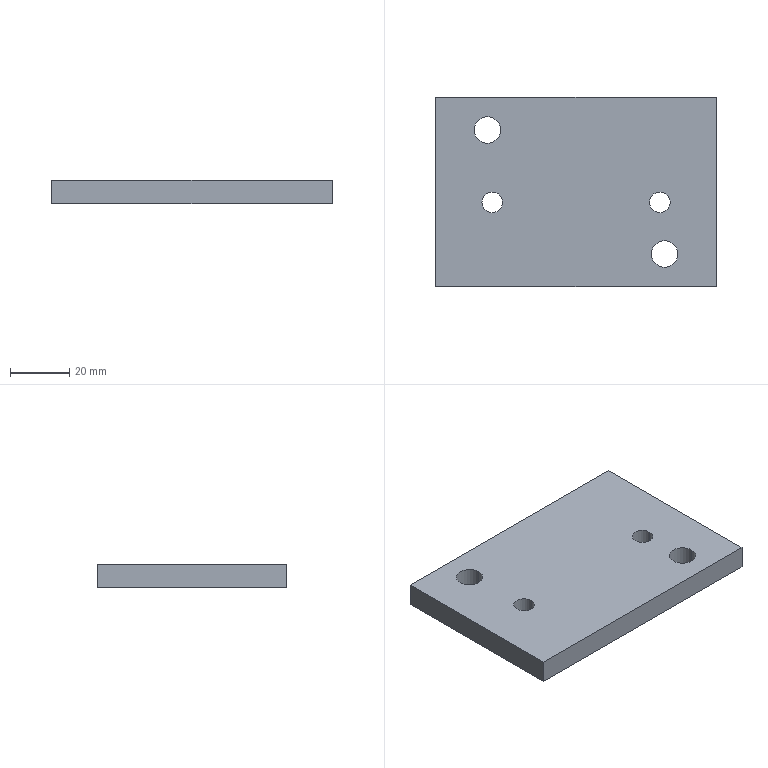Part | 1 solid | 14 faces | box 95 x 64 x 8 mm | volume 47007 mm3 | cylinder 8 | plane 6 | commonest cylinder face diameters 7 x4 9 x4
STEP:
#1=CARTESIAN_POINT('',(0.,0.,0.));
#2=DIRECTION('',(0.,0.,1.));
#3=DIRECTION('',(1.,0.,0.));
#4=AXIS2_PLACEMENT_3D('',#1,#2,#3);
#5=CARTESIAN_POINT('',(-192.5,75.,-105.051));
#6=VERTEX_POINT('',#5);
#7=CARTESIAN_POINT('',(-192.5,139.,-105.051));
#8=VERTEX_POINT('',#7);
#9=CARTESIAN_POINT('',(-192.5,75.,-105.051));
#10=DIRECTION('',(0.,1.,0.));
#11=VECTOR('',#10,1.);
#12=LINE('',#9,#11);
#13=CARTESIAN_POINT('',(-192.5,75.,-113.051));
#14=DIRECTION('',(1.,0.,0.));
#15=DIRECTION('',(0.,0.,1.));
#16=AXIS2_PLACEMENT_3D('',#13,#14,#15);
#17=PLANE('',#16);
#18=CARTESIAN_POINT('',(8.,0.));
#19=DIRECTION('',(0.,-1.));
#20=VECTOR('',#19,1.);
#21=LINE('',#18,#20);
#22=(GEOMETRIC_REPRESENTATION_CONTEXT(2)PARAMETRIC_REPRESENTATION_CONTEXT()REPRESENTATION_CONTEXT('',''));
#23=DEFINITIONAL_REPRESENTATION('',(#21),#22);
#24=PCURVE('',#17,#23);
#25=CARTESIAN_POINT('',(-210.,86.,-105.051));
#26=DIRECTION('',(0.,0.,1.));
#27=DIRECTION('',(-1.,0.,0.));
#28=AXIS2_PLACEMENT_3D('',#25,#26,#27);
#29=PLANE('',#28);
#30=CARTESIAN_POINT('',(-17.5,11.));
#31=DIRECTION('',(0.,-1.));
#32=VECTOR('',#31,1.);
#33=LINE('',#30,#32);
#34=(GEOMETRIC_REPRESENTATION_CONTEXT(2)PARAMETRIC_REPRESENTATION_CONTEXT()REPRESENTATION_CONTEXT('',''));
#35=DEFINITIONAL_REPRESENTATION('',(#33),#34);
#36=PCURVE('',#29,#35);
#37=SURFACE_CURVE('',#12,(#24,#36),.PCURVE_S1.);
#38=EDGE_CURVE('',#6,#8,#37,.T.);
#39=ORIENTED_EDGE('',*,*,#38,.F.);
#40=CARTESIAN_POINT('',(-192.5,75.,-113.051));
#41=VERTEX_POINT('',#40);
#42=CARTESIAN_POINT('',(-192.5,75.,-113.051));
#43=DIRECTION('',(0.,0.,1.));
#44=VECTOR('',#43,1.);
#45=LINE('',#42,#44);
#46=CARTESIAN_POINT('',(0.,0.));
#47=DIRECTION('',(1.,0.));
#48=VECTOR('',#47,1.);
#49=LINE('',#46,#48);
#50=(GEOMETRIC_REPRESENTATION_CONTEXT(2)PARAMETRIC_REPRESENTATION_CONTEXT()REPRESENTATION_CONTEXT('',''));
#51=DEFINITIONAL_REPRESENTATION('',(#49),#50);
#52=PCURVE('',#17,#51);
#53=CARTESIAN_POINT('',(-287.5,75.,-113.051));
#54=DIRECTION('',(0.,-1.,0.));
#55=DIRECTION('',(0.,0.,1.));
#56=AXIS2_PLACEMENT_3D('',#53,#54,#55);
#57=PLANE('',#56);
#58=CARTESIAN_POINT('',(0.,-95.));
#59=DIRECTION('',(1.,0.));
#60=VECTOR('',#59,1.);
#61=LINE('',#58,#60);
#62=(GEOMETRIC_REPRESENTATION_CONTEXT(2)PARAMETRIC_REPRESENTATION_CONTEXT()REPRESENTATION_CONTEXT('',''));
#63=DEFINITIONAL_REPRESENTATION('',(#61),#62);
#64=PCURVE('',#57,#63);
#65=SURFACE_CURVE('',#45,(#52,#64),.PCURVE_S1.);
#66=EDGE_CURVE('',#41,#6,#65,.T.);
#67=ORIENTED_EDGE('',*,*,#66,.F.);
#68=CARTESIAN_POINT('',(-192.5,139.,-113.051));
#69=VERTEX_POINT('',#68);
#70=CARTESIAN_POINT('',(-192.5,75.,-113.051));
#71=DIRECTION('',(0.,1.,0.));
#72=VECTOR('',#71,1.);
#73=LINE('',#70,#72);
#74=CARTESIAN_POINT('',(0.,0.));
#75=DIRECTION('',(0.,-1.));
#76=VECTOR('',#75,1.);
#77=LINE('',#74,#76);
#78=(GEOMETRIC_REPRESENTATION_CONTEXT(2)PARAMETRIC_REPRESENTATION_CONTEXT()REPRESENTATION_CONTEXT('',''));
#79=DEFINITIONAL_REPRESENTATION('',(#77),#78);
#80=PCURVE('',#17,#79);
#81=CARTESIAN_POINT('',(-210.,86.,-113.051));
#82=DIRECTION('',(0.,0.,1.));
#83=DIRECTION('',(-1.,0.,0.));
#84=AXIS2_PLACEMENT_3D('',#81,#82,#83);
#85=PLANE('',#84);
#86=CARTESIAN_POINT('',(-17.5,11.));
#87=DIRECTION('',(0.,-1.));
#88=VECTOR('',#87,1.);
#89=LINE('',#86,#88);
#90=(GEOMETRIC_REPRESENTATION_CONTEXT(2)PARAMETRIC_REPRESENTATION_CONTEXT()REPRESENTATION_CONTEXT('',''));
#91=DEFINITIONAL_REPRESENTATION('',(#89),#90);
#92=PCURVE('',#85,#91);
#93=SURFACE_CURVE('',#73,(#80,#92),.PCURVE_S1.);
#94=EDGE_CURVE('',#41,#69,#93,.T.);
#95=ORIENTED_EDGE('',*,*,#94,.T.);
#96=CARTESIAN_POINT('',(-192.5,139.,-113.051));
#97=DIRECTION('',(0.,0.,1.));
#98=VECTOR('',#97,1.);
#99=LINE('',#96,#98);
#100=CARTESIAN_POINT('',(0.,-64.));
#101=DIRECTION('',(1.,0.));
#102=VECTOR('',#101,1.);
#103=LINE('',#100,#102);
#104=(GEOMETRIC_REPRESENTATION_CONTEXT(2)PARAMETRIC_REPRESENTATION_CONTEXT()REPRESENTATION_CONTEXT('',''));
#105=DEFINITIONAL_REPRESENTATION('',(#103),#104);
#106=PCURVE('',#17,#105);
#107=CARTESIAN_POINT('',(-192.5,139.,-113.051));
#108=DIRECTION('',(0.,1.,0.));
#109=DIRECTION('',(0.,0.,-1.));
#110=AXIS2_PLACEMENT_3D('',#107,#108,#109);
#111=PLANE('',#110);
#112=CARTESIAN_POINT('',(0.,0.));
#113=DIRECTION('',(-1.,0.));
#114=VECTOR('',#113,1.);
#115=LINE('',#112,#114);
#116=(GEOMETRIC_REPRESENTATION_CONTEXT(2)PARAMETRIC_REPRESENTATION_CONTEXT()REPRESENTATION_CONTEXT('',''));
#117=DEFINITIONAL_REPRESENTATION('',(#115),#116);
#118=PCURVE('',#111,#117);
#119=SURFACE_CURVE('',#99,(#106,#118),.PCURVE_S1.);
#120=EDGE_CURVE('',#69,#8,#119,.T.);
#121=ORIENTED_EDGE('',*,*,#120,.T.);
#122=EDGE_LOOP('',(#39,#67,#95,#121));
#123=FACE_BOUND('',#122,.T.);
#124=ADVANCED_FACE('',(#123),#17,.T.);
#125=CARTESIAN_POINT('',(-287.5,139.,-105.051));
#126=VERTEX_POINT('',#125);
#127=CARTESIAN_POINT('',(-192.5,139.,-105.051));
#128=DIRECTION('',(-1.,0.,0.));
#129=VECTOR('',#128,1.);
#130=LINE('',#127,#129);
#131=CARTESIAN_POINT('',(-8.,0.));
#132=DIRECTION('',(0.,1.));
#133=VECTOR('',#132,1.);
#134=LINE('',#131,#133);
#135=(GEOMETRIC_REPRESENTATION_CONTEXT(2)PARAMETRIC_REPRESENTATION_CONTEXT()REPRESENTATION_CONTEXT('',''));
#136=DEFINITIONAL_REPRESENTATION('',(#134),#135);
#137=PCURVE('',#111,#136);
#138=CARTESIAN_POINT('',(-17.5,-53.));
#139=DIRECTION('',(1.,0.));
#140=VECTOR('',#139,1.);
#141=LINE('',#138,#140);
#142=(GEOMETRIC_REPRESENTATION_CONTEXT(2)PARAMETRIC_REPRESENTATION_CONTEXT()REPRESENTATION_CONTEXT('',''));
#143=DEFINITIONAL_REPRESENTATION('',(#141),#142);
#144=PCURVE('',#29,#143);
#145=SURFACE_CURVE('',#130,(#137,#144),.PCURVE_S1.);
#146=EDGE_CURVE('',#8,#126,#145,.T.);
#147=ORIENTED_EDGE('',*,*,#146,.F.);
#148=ORIENTED_EDGE('',*,*,#120,.F.);
#149=CARTESIAN_POINT('',(-287.5,139.,-113.051));
#150=VERTEX_POINT('',#149);
#151=CARTESIAN_POINT('',(-192.5,139.,-113.051));
#152=DIRECTION('',(-1.,0.,0.));
#153=VECTOR('',#152,1.);
#154=LINE('',#151,#153);
#155=CARTESIAN_POINT('',(0.,0.));
#156=DIRECTION('',(0.,1.));
#157=VECTOR('',#156,1.);
#158=LINE('',#155,#157);
#159=(GEOMETRIC_REPRESENTATION_CONTEXT(2)PARAMETRIC_REPRESENTATION_CONTEXT()REPRESENTATION_CONTEXT('',''));
#160=DEFINITIONAL_REPRESENTATION('',(#158),#159);
#161=PCURVE('',#111,#160);
#162=CARTESIAN_POINT('',(-17.5,-53.));
#163=DIRECTION('',(1.,0.));
#164=VECTOR('',#163,1.);
#165=LINE('',#162,#164);
#166=(GEOMETRIC_REPRESENTATION_CONTEXT(2)PARAMETRIC_REPRESENTATION_CONTEXT()REPRESENTATION_CONTEXT('',''));
#167=DEFINITIONAL_REPRESENTATION('',(#165),#166);
#168=PCURVE('',#85,#167);
#169=SURFACE_CURVE('',#154,(#161,#168),.PCURVE_S1.);
#170=EDGE_CURVE('',#69,#150,#169,.T.);
#171=ORIENTED_EDGE('',*,*,#170,.T.);
#172=CARTESIAN_POINT('',(-287.5,139.,-113.051));
#173=DIRECTION('',(0.,0.,1.));
#174=VECTOR('',#173,1.);
#175=LINE('',#172,#174);
#176=CARTESIAN_POINT('',(0.,95.));
#177=DIRECTION('',(-1.,0.));
#178=VECTOR('',#177,1.);
#179=LINE('',#176,#178);
#180=(GEOMETRIC_REPRESENTATION_CONTEXT(2)PARAMETRIC_REPRESENTATION_CONTEXT()REPRESENTATION_CONTEXT('',''));
#181=DEFINITIONAL_REPRESENTATION('',(#179),#180);
#182=PCURVE('',#111,#181);
#183=CARTESIAN_POINT('',(-287.5,139.,-113.051));
#184=DIRECTION('',(-1.,0.,0.));
#185=DIRECTION('',(0.,0.,-1.));
#186=AXIS2_PLACEMENT_3D('',#183,#184,#185);
#187=PLANE('',#186);
#188=CARTESIAN_POINT('',(0.,0.));
#189=DIRECTION('',(-1.,0.));
#190=VECTOR('',#189,1.);
#191=LINE('',#188,#190);
#192=(GEOMETRIC_REPRESENTATION_CONTEXT(2)PARAMETRIC_REPRESENTATION_CONTEXT()REPRESENTATION_CONTEXT('',''));
#193=DEFINITIONAL_REPRESENTATION('',(#191),#192);
#194=PCURVE('',#187,#193);
#195=SURFACE_CURVE('',#175,(#182,#194),.PCURVE_S1.);
#196=EDGE_CURVE('',#150,#126,#195,.T.);
#197=ORIENTED_EDGE('',*,*,#196,.T.);
#198=EDGE_LOOP('',(#147,#148,#171,#197));
#199=FACE_BOUND('',#198,.T.);
#200=ADVANCED_FACE('',(#199),#111,.T.);
#201=CARTESIAN_POINT('',(-287.5,75.,-105.051));
#202=VERTEX_POINT('',#201);
#203=CARTESIAN_POINT('',(-287.5,139.,-105.051));
#204=DIRECTION('',(0.,-1.,0.));
#205=VECTOR('',#204,1.);
#206=LINE('',#203,#205);
#207=CARTESIAN_POINT('',(-8.,0.));
#208=DIRECTION('',(0.,1.));
#209=VECTOR('',#208,1.);
#210=LINE('',#207,#209);
#211=(GEOMETRIC_REPRESENTATION_CONTEXT(2)PARAMETRIC_REPRESENTATION_CONTEXT()REPRESENTATION_CONTEXT('',''));
#212=DEFINITIONAL_REPRESENTATION('',(#210),#211);
#213=PCURVE('',#187,#212);
#214=CARTESIAN_POINT('',(77.5,-53.));
#215=DIRECTION('',(0.,1.));
#216=VECTOR('',#215,1.);
#217=LINE('',#214,#216);
#218=(GEOMETRIC_REPRESENTATION_CONTEXT(2)PARAMETRIC_REPRESENTATION_CONTEXT()REPRESENTATION_CONTEXT('',''));
#219=DEFINITIONAL_REPRESENTATION('',(#217),#218);
#220=PCURVE('',#29,#219);
#221=SURFACE_CURVE('',#206,(#213,#220),.PCURVE_S1.);
#222=EDGE_CURVE('',#126,#202,#221,.T.);
#223=ORIENTED_EDGE('',*,*,#222,.F.);
#224=ORIENTED_EDGE('',*,*,#196,.F.);
#225=CARTESIAN_POINT('',(-287.5,75.,-113.051));
#226=VERTEX_POINT('',#225);
#227=CARTESIAN_POINT('',(-287.5,139.,-113.051));
#228=DIRECTION('',(0.,-1.,0.));
#229=VECTOR('',#228,1.);
#230=LINE('',#227,#229);
#231=CARTESIAN_POINT('',(0.,0.));
#232=DIRECTION('',(0.,1.));
#233=VECTOR('',#232,1.);
#234=LINE('',#231,#233);
#235=(GEOMETRIC_REPRESENTATION_CONTEXT(2)PARAMETRIC_REPRESENTATION_CONTEXT()REPRESENTATION_CONTEXT('',''));
#236=DEFINITIONAL_REPRESENTATION('',(#234),#235);
#237=PCURVE('',#187,#236);
#238=CARTESIAN_POINT('',(77.5,-53.));
#239=DIRECTION('',(0.,1.));
#240=VECTOR('',#239,1.);
#241=LINE('',#238,#240);
#242=(GEOMETRIC_REPRESENTATION_CONTEXT(2)PARAMETRIC_REPRESENTATION_CONTEXT()REPRESENTATION_CONTEXT('',''));
#243=DEFINITIONAL_REPRESENTATION('',(#241),#242);
#244=PCURVE('',#85,#243);
#245=SURFACE_CURVE('',#230,(#237,#244),.PCURVE_S1.);
#246=EDGE_CURVE('',#150,#226,#245,.T.);
#247=ORIENTED_EDGE('',*,*,#246,.T.);
#248=CARTESIAN_POINT('',(-287.5,75.,-113.051));
#249=DIRECTION('',(0.,0.,1.));
#250=VECTOR('',#249,1.);
#251=LINE('',#248,#250);
#252=CARTESIAN_POINT('',(0.,64.));
#253=DIRECTION('',(-1.,0.));
#254=VECTOR('',#253,1.);
#255=LINE('',#252,#254);
#256=(GEOMETRIC_REPRESENTATION_CONTEXT(2)PARAMETRIC_REPRESENTATION_CONTEXT()REPRESENTATION_CONTEXT('',''));
#257=DEFINITIONAL_REPRESENTATION('',(#255),#256);
#258=PCURVE('',#187,#257);
#259=CARTESIAN_POINT('',(0.,0.));
#260=DIRECTION('',(1.,0.));
#261=VECTOR('',#260,1.);
#262=LINE('',#259,#261);
#263=(GEOMETRIC_REPRESENTATION_CONTEXT(2)PARAMETRIC_REPRESENTATION_CONTEXT()REPRESENTATION_CONTEXT('',''));
#264=DEFINITIONAL_REPRESENTATION('',(#262),#263);
#265=PCURVE('',#57,#264);
#266=SURFACE_CURVE('',#251,(#258,#265),.PCURVE_S1.);
#267=EDGE_CURVE('',#226,#202,#266,.T.);
#268=ORIENTED_EDGE('',*,*,#267,.T.);
#269=EDGE_LOOP('',(#223,#224,#247,#268));
#270=FACE_BOUND('',#269,.T.);
#271=ADVANCED_FACE('',(#270),#187,.T.);
#272=CARTESIAN_POINT('',(-287.5,75.,-105.051));
#273=DIRECTION('',(1.,0.,0.));
#274=VECTOR('',#273,1.);
#275=LINE('',#272,#274);
#276=CARTESIAN_POINT('',(8.,0.));
#277=DIRECTION('',(0.,-1.));
#278=VECTOR('',#277,1.);
#279=LINE('',#276,#278);
#280=(GEOMETRIC_REPRESENTATION_CONTEXT(2)PARAMETRIC_REPRESENTATION_CONTEXT()REPRESENTATION_CONTEXT('',''));
#281=DEFINITIONAL_REPRESENTATION('',(#279),#280);
#282=PCURVE('',#57,#281);
#283=CARTESIAN_POINT('',(77.5,11.));
#284=DIRECTION('',(-1.,0.));
#285=VECTOR('',#284,1.);
#286=LINE('',#283,#285);
#287=(GEOMETRIC_REPRESENTATION_CONTEXT(2)PARAMETRIC_REPRESENTATION_CONTEXT()REPRESENTATION_CONTEXT('',''));
#288=DEFINITIONAL_REPRESENTATION('',(#286),#287);
#289=PCURVE('',#29,#288);
#290=SURFACE_CURVE('',#275,(#282,#289),.PCURVE_S1.);
#291=EDGE_CURVE('',#202,#6,#290,.T.);
#292=ORIENTED_EDGE('',*,*,#291,.F.);
#293=ORIENTED_EDGE('',*,*,#267,.F.);
#294=CARTESIAN_POINT('',(-287.5,75.,-113.051));
#295=DIRECTION('',(1.,0.,0.));
#296=VECTOR('',#295,1.);
#297=LINE('',#294,#296);
#298=CARTESIAN_POINT('',(0.,0.));
#299=DIRECTION('',(0.,-1.));
#300=VECTOR('',#299,1.);
#301=LINE('',#298,#300);
#302=(GEOMETRIC_REPRESENTATION_CONTEXT(2)PARAMETRIC_REPRESENTATION_CONTEXT()REPRESENTATION_CONTEXT('',''));
#303=DEFINITIONAL_REPRESENTATION('',(#301),#302);
#304=PCURVE('',#57,#303);
#305=CARTESIAN_POINT('',(77.5,11.));
#306=DIRECTION('',(-1.,0.));
#307=VECTOR('',#306,1.);
#308=LINE('',#305,#307);
#309=(GEOMETRIC_REPRESENTATION_CONTEXT(2)PARAMETRIC_REPRESENTATION_CONTEXT()REPRESENTATION_CONTEXT('',''));
#310=DEFINITIONAL_REPRESENTATION('',(#308),#309);
#311=PCURVE('',#85,#310);
#312=SURFACE_CURVE('',#297,(#304,#311),.PCURVE_S1.);
#313=EDGE_CURVE('',#226,#41,#312,.T.);
#314=ORIENTED_EDGE('',*,*,#313,.T.);
#315=ORIENTED_EDGE('',*,*,#66,.T.);
#316=EDGE_LOOP('',(#292,#293,#314,#315));
#317=FACE_BOUND('',#316,.T.);
#318=ADVANCED_FACE('',(#317),#57,.T.);
#319=ORIENTED_EDGE('',*,*,#94,.F.);
#320=ORIENTED_EDGE('',*,*,#313,.F.);
#321=ORIENTED_EDGE('',*,*,#246,.F.);
#322=ORIENTED_EDGE('',*,*,#170,.F.);
#323=EDGE_LOOP('',(#319,#320,#321,#322));
#324=FACE_BOUND('',#323,.T.);
#325=CARTESIAN_POINT('',(-214.5,86.,-113.051));
#326=VERTEX_POINT('',#325);
#327=CARTESIAN_POINT('',(-205.5,86.,-113.051));
#328=VERTEX_POINT('',#327);
#329=CARTESIAN_POINT('',(-210.,86.,-113.051));
#330=DIRECTION('',(0.,0.,1.));
#331=DIRECTION('',(-1.,0.,0.));
#332=AXIS2_PLACEMENT_3D('',#329,#330,#331);
#333=CIRCLE('',#332,4.5);
#334=CARTESIAN_POINT('',(0.,0.));
#335=DIRECTION('',(1.,0.));
#336=AXIS2_PLACEMENT_2D('',#334,#335);
#337=CIRCLE('',#336,4.5);
#338=(GEOMETRIC_REPRESENTATION_CONTEXT(2)PARAMETRIC_REPRESENTATION_CONTEXT()REPRESENTATION_CONTEXT('',''));
#339=DEFINITIONAL_REPRESENTATION('',(#337),#338);
#340=PCURVE('',#85,#339);
#341=CARTESIAN_POINT('',(-210.,86.,-113.051));
#342=DIRECTION('',(0.,0.,1.));
#343=DIRECTION('',(0.,1.,0.));
#344=AXIS2_PLACEMENT_3D('',#341,#342,#343);
#345=CYLINDRICAL_SURFACE('',#344,4.5);
#346=CARTESIAN_POINT('',(1.571,0.));
#347=DIRECTION('',(1.,0.));
#348=VECTOR('',#347,1.);
#349=LINE('',#346,#348);
#350=(GEOMETRIC_REPRESENTATION_CONTEXT(2)PARAMETRIC_REPRESENTATION_CONTEXT()REPRESENTATION_CONTEXT('',''));
#351=DEFINITIONAL_REPRESENTATION('',(#349),#350);
#352=PCURVE('',#345,#351);
#353=SURFACE_CURVE('',#333,(#340,#352),.PCURVE_S1.);
#354=EDGE_CURVE('',#326,#328,#353,.T.);
#355=ORIENTED_EDGE('',*,*,#354,.T.);
#356=CARTESIAN_POINT('',(-210.,86.,-113.051));
#357=DIRECTION('',(0.,0.,1.));
#358=DIRECTION('',(-1.,0.,0.));
#359=AXIS2_PLACEMENT_3D('',#356,#357,#358);
#360=CIRCLE('',#359,4.5);
#361=CARTESIAN_POINT('',(0.,0.));
#362=DIRECTION('',(1.,0.));
#363=AXIS2_PLACEMENT_2D('',#361,#362);
#364=CIRCLE('',#363,4.5);
#365=(GEOMETRIC_REPRESENTATION_CONTEXT(2)PARAMETRIC_REPRESENTATION_CONTEXT()REPRESENTATION_CONTEXT('',''));
#366=DEFINITIONAL_REPRESENTATION('',(#364),#365);
#367=PCURVE('',#85,#366);
#368=CARTESIAN_POINT('',(-210.,86.,-113.051));
#369=DIRECTION('',(0.,0.,1.));
#370=DIRECTION('',(0.,-1.,0.));
#371=AXIS2_PLACEMENT_3D('',#368,#369,#370);
#372=CYLINDRICAL_SURFACE('',#371,4.5);
#373=CARTESIAN_POINT('',(-1.571,0.));
#374=DIRECTION('',(1.,0.));
#375=VECTOR('',#374,1.);
#376=LINE('',#373,#375);
#377=(GEOMETRIC_REPRESENTATION_CONTEXT(2)PARAMETRIC_REPRESENTATION_CONTEXT()REPRESENTATION_CONTEXT('',''));
#378=DEFINITIONAL_REPRESENTATION('',(#376),#377);
#379=PCURVE('',#372,#378);
#380=SURFACE_CURVE('',#360,(#367,#379),.PCURVE_S1.);
#381=EDGE_CURVE('',#328,#326,#380,.T.);
#382=ORIENTED_EDGE('',*,*,#381,.T.);
#383=EDGE_LOOP('',(#355,#382));
#384=FACE_BOUND('',#383,.T.);
#385=CARTESIAN_POINT('',(-271.863,103.5,-113.051));
#386=VERTEX_POINT('',#385);
#387=CARTESIAN_POINT('',(-264.863,103.5,-113.051));
#388=VERTEX_POINT('',#387);
#389=CARTESIAN_POINT('',(-268.363,103.5,-113.051));
#390=DIRECTION('',(0.,0.,1.));
#391=DIRECTION('',(-1.,0.,0.));
#392=AXIS2_PLACEMENT_3D('',#389,#390,#391);
#393=CIRCLE('',#392,3.5);
#394=CARTESIAN_POINT('',(58.363,-17.5));
#395=DIRECTION('',(1.,0.));
#396=AXIS2_PLACEMENT_2D('',#394,#395);
#397=CIRCLE('',#396,3.5);
#398=(GEOMETRIC_REPRESENTATION_CONTEXT(2)PARAMETRIC_REPRESENTATION_CONTEXT()REPRESENTATION_CONTEXT('',''));
#399=DEFINITIONAL_REPRESENTATION('',(#397),#398);
#400=PCURVE('',#85,#399);
#401=CARTESIAN_POINT('',(-268.363,103.5,-113.051));
#402=DIRECTION('',(0.,0.,1.));
#403=DIRECTION('',(0.,1.,0.));
#404=AXIS2_PLACEMENT_3D('',#401,#402,#403);
#405=CYLINDRICAL_SURFACE('',#404,3.5);
#406=CARTESIAN_POINT('',(1.571,0.));
#407=DIRECTION('',(1.,0.));
#408=VECTOR('',#407,1.);
#409=LINE('',#406,#408);
#410=(GEOMETRIC_REPRESENTATION_CONTEXT(2)PARAMETRIC_REPRESENTATION_CONTEXT()REPRESENTATION_CONTEXT('',''));
#411=DEFINITIONAL_REPRESENTATION('',(#409),#410);
#412=PCURVE('',#405,#411);
#413=SURFACE_CURVE('',#393,(#400,#412),.PCURVE_S1.);
#414=EDGE_CURVE('',#386,#388,#413,.T.);
#415=ORIENTED_EDGE('',*,*,#414,.T.);
#416=CARTESIAN_POINT('',(-268.363,103.5,-113.051));
#417=DIRECTION('',(0.,0.,1.));
#418=DIRECTION('',(-1.,0.,0.));
#419=AXIS2_PLACEMENT_3D('',#416,#417,#418);
#420=CIRCLE('',#419,3.5);
#421=CARTESIAN_POINT('',(58.363,-17.5));
#422=DIRECTION('',(1.,0.));
#423=AXIS2_PLACEMENT_2D('',#421,#422);
#424=CIRCLE('',#423,3.5);
#425=(GEOMETRIC_REPRESENTATION_CONTEXT(2)PARAMETRIC_REPRESENTATION_CONTEXT()REPRESENTATION_CONTEXT('',''));
#426=DEFINITIONAL_REPRESENTATION('',(#424),#425);
#427=PCURVE('',#85,#426);
#428=CARTESIAN_POINT('',(-268.363,103.5,-113.051));
#429=DIRECTION('',(0.,0.,1.));
#430=DIRECTION('',(0.,-1.,0.));
#431=AXIS2_PLACEMENT_3D('',#428,#429,#430);
#432=CYLINDRICAL_SURFACE('',#431,3.5);
#433=CARTESIAN_POINT('',(-1.571,0.));
#434=DIRECTION('',(1.,0.));
#435=VECTOR('',#434,1.);
#436=LINE('',#433,#435);
#437=(GEOMETRIC_REPRESENTATION_CONTEXT(2)PARAMETRIC_REPRESENTATION_CONTEXT()REPRESENTATION_CONTEXT('',''));
#438=DEFINITIONAL_REPRESENTATION('',(#436),#437);
#439=PCURVE('',#432,#438);
#440=SURFACE_CURVE('',#420,(#427,#439),.PCURVE_S1.);
#441=EDGE_CURVE('',#388,#386,#440,.T.);
#442=ORIENTED_EDGE('',*,*,#441,.T.);
#443=EDGE_LOOP('',(#415,#442));
#444=FACE_BOUND('',#443,.T.);
#445=CARTESIAN_POINT('',(-274.5,128.,-113.051));
#446=VERTEX_POINT('',#445);
#447=CARTESIAN_POINT('',(-265.5,128.,-113.051));
#448=VERTEX_POINT('',#447);
#449=CARTESIAN_POINT('',(-270.,128.,-113.051));
#450=DIRECTION('',(0.,0.,1.));
#451=DIRECTION('',(-1.,0.,0.));
#452=AXIS2_PLACEMENT_3D('',#449,#450,#451);
#453=CIRCLE('',#452,4.5);
#454=CARTESIAN_POINT('',(60.,-42.));
#455=DIRECTION('',(1.,0.));
#456=AXIS2_PLACEMENT_2D('',#454,#455);
#457=CIRCLE('',#456,4.5);
#458=(GEOMETRIC_REPRESENTATION_CONTEXT(2)PARAMETRIC_REPRESENTATION_CONTEXT()REPRESENTATION_CONTEXT('',''));
#459=DEFINITIONAL_REPRESENTATION('',(#457),#458);
#460=PCURVE('',#85,#459);
#461=CARTESIAN_POINT('',(-270.,128.,-113.051));
#462=DIRECTION('',(0.,0.,1.));
#463=DIRECTION('',(0.,1.,0.));
#464=AXIS2_PLACEMENT_3D('',#461,#462,#463);
#465=CYLINDRICAL_SURFACE('',#464,4.5);
#466=CARTESIAN_POINT('',(1.571,0.));
#467=DIRECTION('',(1.,0.));
#468=VECTOR('',#467,1.);
#469=LINE('',#466,#468);
#470=(GEOMETRIC_REPRESENTATION_CONTEXT(2)PARAMETRIC_REPRESENTATION_CONTEXT()REPRESENTATION_CONTEXT('',''));
#471=DEFINITIONAL_REPRESENTATION('',(#469),#470);
#472=PCURVE('',#465,#471);
#473=SURFACE_CURVE('',#453,(#460,#472),.PCURVE_S1.);
#474=EDGE_CURVE('',#446,#448,#473,.T.);
#475=ORIENTED_EDGE('',*,*,#474,.T.);
#476=CARTESIAN_POINT('',(-270.,128.,-113.051));
#477=DIRECTION('',(0.,0.,1.));
#478=DIRECTION('',(-1.,0.,0.));
#479=AXIS2_PLACEMENT_3D('',#476,#477,#478);
#480=CIRCLE('',#479,4.5);
#481=CARTESIAN_POINT('',(60.,-42.));
#482=DIRECTION('',(1.,0.));
#483=AXIS2_PLACEMENT_2D('',#481,#482);
#484=CIRCLE('',#483,4.5);
#485=(GEOMETRIC_REPRESENTATION_CONTEXT(2)PARAMETRIC_REPRESENTATION_CONTEXT()REPRESENTATION_CONTEXT('',''));
#486=DEFINITIONAL_REPRESENTATION('',(#484),#485);
#487=PCURVE('',#85,#486);
#488=CARTESIAN_POINT('',(-270.,128.,-113.051));
#489=DIRECTION('',(0.,0.,1.));
#490=DIRECTION('',(0.,-1.,0.));
#491=AXIS2_PLACEMENT_3D('',#488,#489,#490);
#492=CYLINDRICAL_SURFACE('',#491,4.5);
#493=CARTESIAN_POINT('',(-1.571,0.));
#494=DIRECTION('',(1.,0.));
#495=VECTOR('',#494,1.);
#496=LINE('',#493,#495);
#497=(GEOMETRIC_REPRESENTATION_CONTEXT(2)PARAMETRIC_REPRESENTATION_CONTEXT()REPRESENTATION_CONTEXT('',''));
#498=DEFINITIONAL_REPRESENTATION('',(#496),#497);
#499=PCURVE('',#492,#498);
#500=SURFACE_CURVE('',#480,(#487,#499),.PCURVE_S1.);
#501=EDGE_CURVE('',#448,#446,#500,.T.);
#502=ORIENTED_EDGE('',*,*,#501,.T.);
#503=EDGE_LOOP('',(#475,#502));
#504=FACE_BOUND('',#503,.T.);
#505=CARTESIAN_POINT('',(-215.113,103.5,-113.051));
#506=VERTEX_POINT('',#505);
#507=CARTESIAN_POINT('',(-208.113,103.5,-113.051));
#508=VERTEX_POINT('',#507);
#509=CARTESIAN_POINT('',(-211.613,103.5,-113.051));
#510=DIRECTION('',(0.,0.,1.));
#511=DIRECTION('',(-1.,0.,0.));
#512=AXIS2_PLACEMENT_3D('',#509,#510,#511);
#513=CIRCLE('',#512,3.5);
#514=CARTESIAN_POINT('',(1.613,-17.5));
#515=DIRECTION('',(1.,0.));
#516=AXIS2_PLACEMENT_2D('',#514,#515);
#517=CIRCLE('',#516,3.5);
#518=(GEOMETRIC_REPRESENTATION_CONTEXT(2)PARAMETRIC_REPRESENTATION_CONTEXT()REPRESENTATION_CONTEXT('',''));
#519=DEFINITIONAL_REPRESENTATION('',(#517),#518);
#520=PCURVE('',#85,#519);
#521=CARTESIAN_POINT('',(-211.613,103.5,-113.051));
#522=DIRECTION('',(0.,0.,1.));
#523=DIRECTION('',(0.,1.,0.));
#524=AXIS2_PLACEMENT_3D('',#521,#522,#523);
#525=CYLINDRICAL_SURFACE('',#524,3.5);
#526=CARTESIAN_POINT('',(1.571,0.));
#527=DIRECTION('',(1.,0.));
#528=VECTOR('',#527,1.);
#529=LINE('',#526,#528);
#530=(GEOMETRIC_REPRESENTATION_CONTEXT(2)PARAMETRIC_REPRESENTATION_CONTEXT()REPRESENTATION_CONTEXT('',''));
#531=DEFINITIONAL_REPRESENTATION('',(#529),#530);
#532=PCURVE('',#525,#531);
#533=SURFACE_CURVE('',#513,(#520,#532),.PCURVE_S1.);
#534=EDGE_CURVE('',#506,#508,#533,.T.);
#535=ORIENTED_EDGE('',*,*,#534,.T.);
#536=CARTESIAN_POINT('',(-211.613,103.5,-113.051));
#537=DIRECTION('',(0.,0.,1.));
#538=DIRECTION('',(-1.,0.,0.));
#539=AXIS2_PLACEMENT_3D('',#536,#537,#538);
#540=CIRCLE('',#539,3.5);
#541=CARTESIAN_POINT('',(1.613,-17.5));
#542=DIRECTION('',(1.,0.));
#543=AXIS2_PLACEMENT_2D('',#541,#542);
#544=CIRCLE('',#543,3.5);
#545=(GEOMETRIC_REPRESENTATION_CONTEXT(2)PARAMETRIC_REPRESENTATION_CONTEXT()REPRESENTATION_CONTEXT('',''));
#546=DEFINITIONAL_REPRESENTATION('',(#544),#545);
#547=PCURVE('',#85,#546);
#548=CARTESIAN_POINT('',(-211.613,103.5,-113.051));
#549=DIRECTION('',(0.,0.,1.));
#550=DIRECTION('',(0.,-1.,0.));
#551=AXIS2_PLACEMENT_3D('',#548,#549,#550);
#552=CYLINDRICAL_SURFACE('',#551,3.5);
#553=CARTESIAN_POINT('',(-1.571,0.));
#554=DIRECTION('',(1.,0.));
#555=VECTOR('',#554,1.);
#556=LINE('',#553,#555);
#557=(GEOMETRIC_REPRESENTATION_CONTEXT(2)PARAMETRIC_REPRESENTATION_CONTEXT()REPRESENTATION_CONTEXT('',''));
#558=DEFINITIONAL_REPRESENTATION('',(#556),#557);
#559=PCURVE('',#552,#558);
#560=SURFACE_CURVE('',#540,(#547,#559),.PCURVE_S1.);
#561=EDGE_CURVE('',#508,#506,#560,.T.);
#562=ORIENTED_EDGE('',*,*,#561,.T.);
#563=EDGE_LOOP('',(#535,#562));
#564=FACE_BOUND('',#563,.T.);
#565=ADVANCED_FACE('',(#324,#384,#444,#504,#564),#85,.F.);
#566=ORIENTED_EDGE('',*,*,#561,.T.);
#567=CARTESIAN_POINT('',(-215.113,103.5,-105.051));
#568=VERTEX_POINT('',#567);
#569=CARTESIAN_POINT('',(-215.113,103.5,-113.051));
#570=DIRECTION('',(0.,0.,1.));
#571=VECTOR('',#570,1.);
#572=LINE('',#569,#571);
#573=CARTESIAN_POINT('',(4.712,0.));
#574=DIRECTION('',(0.,1.));
#575=VECTOR('',#574,1.);
#576=LINE('',#573,#575);
#577=(GEOMETRIC_REPRESENTATION_CONTEXT(2)PARAMETRIC_REPRESENTATION_CONTEXT()REPRESENTATION_CONTEXT('',''));
#578=DEFINITIONAL_REPRESENTATION('',(#576),#577);
#579=PCURVE('',#552,#578);
#580=CARTESIAN_POINT('',(1.571,0.));
#581=DIRECTION('',(0.,1.));
#582=VECTOR('',#581,1.);
#583=LINE('',#580,#582);
#584=(GEOMETRIC_REPRESENTATION_CONTEXT(2)PARAMETRIC_REPRESENTATION_CONTEXT()REPRESENTATION_CONTEXT('',''));
#585=DEFINITIONAL_REPRESENTATION('',(#583),#584);
#586=PCURVE('',#525,#585);
#587=SURFACE_CURVE('',#572,(#579,#586),.PCURVE_S1.);
#588=EDGE_CURVE('',#506,#568,#587,.T.);
#589=ORIENTED_EDGE('',*,*,#588,.T.);
#590=CARTESIAN_POINT('',(-208.113,103.5,-105.051));
#591=VERTEX_POINT('',#590);
#592=CARTESIAN_POINT('',(-211.613,103.5,-105.051));
#593=DIRECTION('',(0.,0.,1.));
#594=DIRECTION('',(-1.,0.,0.));
#595=AXIS2_PLACEMENT_3D('',#592,#593,#594);
#596=CIRCLE('',#595,3.5);
#597=CARTESIAN_POINT('',(-1.571,8.));
#598=DIRECTION('',(1.,0.));
#599=VECTOR('',#598,1.);
#600=LINE('',#597,#599);
#601=(GEOMETRIC_REPRESENTATION_CONTEXT(2)PARAMETRIC_REPRESENTATION_CONTEXT()REPRESENTATION_CONTEXT('',''));
#602=DEFINITIONAL_REPRESENTATION('',(#600),#601);
#603=PCURVE('',#552,#602);
#604=CARTESIAN_POINT('',(1.613,-17.5));
#605=DIRECTION('',(1.,0.));
#606=AXIS2_PLACEMENT_2D('',#604,#605);
#607=CIRCLE('',#606,3.5);
#608=(GEOMETRIC_REPRESENTATION_CONTEXT(2)PARAMETRIC_REPRESENTATION_CONTEXT()REPRESENTATION_CONTEXT('',''));
#609=DEFINITIONAL_REPRESENTATION('',(#607),#608);
#610=PCURVE('',#29,#609);
#611=SURFACE_CURVE('',#596,(#603,#610),.PCURVE_S1.);
#612=EDGE_CURVE('',#591,#568,#611,.T.);
#613=ORIENTED_EDGE('',*,*,#612,.F.);
#614=CARTESIAN_POINT('',(-208.113,103.5,-113.051));
#615=DIRECTION('',(0.,0.,1.));
#616=VECTOR('',#615,1.);
#617=LINE('',#614,#616);
#618=CARTESIAN_POINT('',(1.571,0.));
#619=DIRECTION('',(0.,1.));
#620=VECTOR('',#619,1.);
#621=LINE('',#618,#620);
#622=(GEOMETRIC_REPRESENTATION_CONTEXT(2)PARAMETRIC_REPRESENTATION_CONTEXT()REPRESENTATION_CONTEXT('',''));
#623=DEFINITIONAL_REPRESENTATION('',(#621),#622);
#624=PCURVE('',#552,#623);
#625=CARTESIAN_POINT('',(4.712,0.));
#626=DIRECTION('',(0.,1.));
#627=VECTOR('',#626,1.);
#628=LINE('',#625,#627);
#629=(GEOMETRIC_REPRESENTATION_CONTEXT(2)PARAMETRIC_REPRESENTATION_CONTEXT()REPRESENTATION_CONTEXT('',''));
#630=DEFINITIONAL_REPRESENTATION('',(#628),#629);
#631=PCURVE('',#525,#630);
#632=SURFACE_CURVE('',#617,(#624,#631),.PCURVE_S1.);
#633=EDGE_CURVE('',#508,#591,#632,.T.);
#634=ORIENTED_EDGE('',*,*,#633,.F.);
#635=EDGE_LOOP('',(#566,#589,#613,#634));
#636=FACE_BOUND('',#635,.F.);
#637=ADVANCED_FACE('',(#636),#552,.F.);
#638=ORIENTED_EDGE('',*,*,#38,.T.);
#639=ORIENTED_EDGE('',*,*,#146,.T.);
#640=ORIENTED_EDGE('',*,*,#222,.T.);
#641=ORIENTED_EDGE('',*,*,#291,.T.);
#642=EDGE_LOOP('',(#638,#639,#640,#641));
#643=FACE_BOUND('',#642,.T.);
#644=CARTESIAN_POINT('',(-205.5,86.,-105.051));
#645=VERTEX_POINT('',#644);
#646=CARTESIAN_POINT('',(-214.5,86.,-105.051));
#647=VERTEX_POINT('',#646);
#648=CARTESIAN_POINT('',(-210.,86.,-105.051));
#649=DIRECTION('',(0.,0.,1.));
#650=DIRECTION('',(-1.,0.,0.));
#651=AXIS2_PLACEMENT_3D('',#648,#649,#650);
#652=CIRCLE('',#651,4.5);
#653=CARTESIAN_POINT('',(0.,0.));
#654=DIRECTION('',(1.,0.));
#655=AXIS2_PLACEMENT_2D('',#653,#654);
#656=CIRCLE('',#655,4.5);
#657=(GEOMETRIC_REPRESENTATION_CONTEXT(2)PARAMETRIC_REPRESENTATION_CONTEXT()REPRESENTATION_CONTEXT('',''));
#658=DEFINITIONAL_REPRESENTATION('',(#656),#657);
#659=PCURVE('',#29,#658);
#660=CARTESIAN_POINT('',(-1.571,8.));
#661=DIRECTION('',(1.,0.));
#662=VECTOR('',#661,1.);
#663=LINE('',#660,#662);
#664=(GEOMETRIC_REPRESENTATION_CONTEXT(2)PARAMETRIC_REPRESENTATION_CONTEXT()REPRESENTATION_CONTEXT('',''));
#665=DEFINITIONAL_REPRESENTATION('',(#663),#664);
#666=PCURVE('',#372,#665);
#667=SURFACE_CURVE('',#652,(#659,#666),.PCURVE_S1.);
#668=EDGE_CURVE('',#645,#647,#667,.T.);
#669=ORIENTED_EDGE('',*,*,#668,.F.);
#670=CARTESIAN_POINT('',(-210.,86.,-105.051));
#671=DIRECTION('',(0.,0.,1.));
#672=DIRECTION('',(-1.,0.,0.));
#673=AXIS2_PLACEMENT_3D('',#670,#671,#672);
#674=CIRCLE('',#673,4.5);
#675=CARTESIAN_POINT('',(0.,0.));
#676=DIRECTION('',(1.,0.));
#677=AXIS2_PLACEMENT_2D('',#675,#676);
#678=CIRCLE('',#677,4.5);
#679=(GEOMETRIC_REPRESENTATION_CONTEXT(2)PARAMETRIC_REPRESENTATION_CONTEXT()REPRESENTATION_CONTEXT('',''));
#680=DEFINITIONAL_REPRESENTATION('',(#678),#679);
#681=PCURVE('',#29,#680);
#682=CARTESIAN_POINT('',(1.571,8.));
#683=DIRECTION('',(1.,0.));
#684=VECTOR('',#683,1.);
#685=LINE('',#682,#684);
#686=(GEOMETRIC_REPRESENTATION_CONTEXT(2)PARAMETRIC_REPRESENTATION_CONTEXT()REPRESENTATION_CONTEXT('',''));
#687=DEFINITIONAL_REPRESENTATION('',(#685),#686);
#688=PCURVE('',#345,#687);
#689=SURFACE_CURVE('',#674,(#681,#688),.PCURVE_S1.);
#690=EDGE_CURVE('',#647,#645,#689,.T.);
#691=ORIENTED_EDGE('',*,*,#690,.F.);
#692=EDGE_LOOP('',(#669,#691));
#693=FACE_BOUND('',#692,.T.);
#694=CARTESIAN_POINT('',(-264.863,103.5,-105.051));
#695=VERTEX_POINT('',#694);
#696=CARTESIAN_POINT('',(-271.863,103.5,-105.051));
#697=VERTEX_POINT('',#696);
#698=CARTESIAN_POINT('',(-268.363,103.5,-105.051));
#699=DIRECTION('',(0.,0.,1.));
#700=DIRECTION('',(-1.,0.,0.));
#701=AXIS2_PLACEMENT_3D('',#698,#699,#700);
#702=CIRCLE('',#701,3.5);
#703=CARTESIAN_POINT('',(58.363,-17.5));
#704=DIRECTION('',(1.,0.));
#705=AXIS2_PLACEMENT_2D('',#703,#704);
#706=CIRCLE('',#705,3.5);
#707=(GEOMETRIC_REPRESENTATION_CONTEXT(2)PARAMETRIC_REPRESENTATION_CONTEXT()REPRESENTATION_CONTEXT('',''));
#708=DEFINITIONAL_REPRESENTATION('',(#706),#707);
#709=PCURVE('',#29,#708);
#710=CARTESIAN_POINT('',(-1.571,8.));
#711=DIRECTION('',(1.,0.));
#712=VECTOR('',#711,1.);
#713=LINE('',#710,#712);
#714=(GEOMETRIC_REPRESENTATION_CONTEXT(2)PARAMETRIC_REPRESENTATION_CONTEXT()REPRESENTATION_CONTEXT('',''));
#715=DEFINITIONAL_REPRESENTATION('',(#713),#714);
#716=PCURVE('',#432,#715);
#717=SURFACE_CURVE('',#702,(#709,#716),.PCURVE_S1.);
#718=EDGE_CURVE('',#695,#697,#717,.T.);
#719=ORIENTED_EDGE('',*,*,#718,.F.);
#720=CARTESIAN_POINT('',(-268.363,103.5,-105.051));
#721=DIRECTION('',(0.,0.,1.));
#722=DIRECTION('',(-1.,0.,0.));
#723=AXIS2_PLACEMENT_3D('',#720,#721,#722);
#724=CIRCLE('',#723,3.5);
#725=CARTESIAN_POINT('',(58.363,-17.5));
#726=DIRECTION('',(1.,0.));
#727=AXIS2_PLACEMENT_2D('',#725,#726);
#728=CIRCLE('',#727,3.5);
#729=(GEOMETRIC_REPRESENTATION_CONTEXT(2)PARAMETRIC_REPRESENTATION_CONTEXT()REPRESENTATION_CONTEXT('',''));
#730=DEFINITIONAL_REPRESENTATION('',(#728),#729);
#731=PCURVE('',#29,#730);
#732=CARTESIAN_POINT('',(1.571,8.));
#733=DIRECTION('',(1.,0.));
#734=VECTOR('',#733,1.);
#735=LINE('',#732,#734);
#736=(GEOMETRIC_REPRESENTATION_CONTEXT(2)PARAMETRIC_REPRESENTATION_CONTEXT()REPRESENTATION_CONTEXT('',''));
#737=DEFINITIONAL_REPRESENTATION('',(#735),#736);
#738=PCURVE('',#405,#737);
#739=SURFACE_CURVE('',#724,(#731,#738),.PCURVE_S1.);
#740=EDGE_CURVE('',#697,#695,#739,.T.);
#741=ORIENTED_EDGE('',*,*,#740,.F.);
#742=EDGE_LOOP('',(#719,#741));
#743=FACE_BOUND('',#742,.T.);
#744=CARTESIAN_POINT('',(-265.5,128.,-105.051));
#745=VERTEX_POINT('',#744);
#746=CARTESIAN_POINT('',(-274.5,128.,-105.051));
#747=VERTEX_POINT('',#746);
#748=CARTESIAN_POINT('',(-270.,128.,-105.051));
#749=DIRECTION('',(0.,0.,1.));
#750=DIRECTION('',(-1.,0.,0.));
#751=AXIS2_PLACEMENT_3D('',#748,#749,#750);
#752=CIRCLE('',#751,4.5);
#753=CARTESIAN_POINT('',(60.,-42.));
#754=DIRECTION('',(1.,0.));
#755=AXIS2_PLACEMENT_2D('',#753,#754);
#756=CIRCLE('',#755,4.5);
#757=(GEOMETRIC_REPRESENTATION_CONTEXT(2)PARAMETRIC_REPRESENTATION_CONTEXT()REPRESENTATION_CONTEXT('',''));
#758=DEFINITIONAL_REPRESENTATION('',(#756),#757);
#759=PCURVE('',#29,#758);
#760=CARTESIAN_POINT('',(-1.571,8.));
#761=DIRECTION('',(1.,0.));
#762=VECTOR('',#761,1.);
#763=LINE('',#760,#762);
#764=(GEOMETRIC_REPRESENTATION_CONTEXT(2)PARAMETRIC_REPRESENTATION_CONTEXT()REPRESENTATION_CONTEXT('',''));
#765=DEFINITIONAL_REPRESENTATION('',(#763),#764);
#766=PCURVE('',#492,#765);
#767=SURFACE_CURVE('',#752,(#759,#766),.PCURVE_S1.);
#768=EDGE_CURVE('',#745,#747,#767,.T.);
#769=ORIENTED_EDGE('',*,*,#768,.F.);
#770=CARTESIAN_POINT('',(-270.,128.,-105.051));
#771=DIRECTION('',(0.,0.,1.));
#772=DIRECTION('',(-1.,0.,0.));
#773=AXIS2_PLACEMENT_3D('',#770,#771,#772);
#774=CIRCLE('',#773,4.5);
#775=CARTESIAN_POINT('',(60.,-42.));
#776=DIRECTION('',(1.,0.));
#777=AXIS2_PLACEMENT_2D('',#775,#776);
#778=CIRCLE('',#777,4.5);
#779=(GEOMETRIC_REPRESENTATION_CONTEXT(2)PARAMETRIC_REPRESENTATION_CONTEXT()REPRESENTATION_CONTEXT('',''));
#780=DEFINITIONAL_REPRESENTATION('',(#778),#779);
#781=PCURVE('',#29,#780);
#782=CARTESIAN_POINT('',(1.571,8.));
#783=DIRECTION('',(1.,0.));
#784=VECTOR('',#783,1.);
#785=LINE('',#782,#784);
#786=(GEOMETRIC_REPRESENTATION_CONTEXT(2)PARAMETRIC_REPRESENTATION_CONTEXT()REPRESENTATION_CONTEXT('',''));
#787=DEFINITIONAL_REPRESENTATION('',(#785),#786);
#788=PCURVE('',#465,#787);
#789=SURFACE_CURVE('',#774,(#781,#788),.PCURVE_S1.);
#790=EDGE_CURVE('',#747,#745,#789,.T.);
#791=ORIENTED_EDGE('',*,*,#790,.F.);
#792=EDGE_LOOP('',(#769,#791));
#793=FACE_BOUND('',#792,.T.);
#794=ORIENTED_EDGE('',*,*,#612,.F.);
#795=CARTESIAN_POINT('',(-211.613,103.5,-105.051));
#796=DIRECTION('',(0.,0.,1.));
#797=DIRECTION('',(-1.,0.,0.));
#798=AXIS2_PLACEMENT_3D('',#795,#796,#797);
#799=CIRCLE('',#798,3.5);
#800=CARTESIAN_POINT('',(1.613,-17.5));
#801=DIRECTION('',(1.,0.));
#802=AXIS2_PLACEMENT_2D('',#800,#801);
#803=CIRCLE('',#802,3.5);
#804=(GEOMETRIC_REPRESENTATION_CONTEXT(2)PARAMETRIC_REPRESENTATION_CONTEXT()REPRESENTATION_CONTEXT('',''));
#805=DEFINITIONAL_REPRESENTATION('',(#803),#804);
#806=PCURVE('',#29,#805);
#807=CARTESIAN_POINT('',(1.571,8.));
#808=DIRECTION('',(1.,0.));
#809=VECTOR('',#808,1.);
#810=LINE('',#807,#809);
#811=(GEOMETRIC_REPRESENTATION_CONTEXT(2)PARAMETRIC_REPRESENTATION_CONTEXT()REPRESENTATION_CONTEXT('',''));
#812=DEFINITIONAL_REPRESENTATION('',(#810),#811);
#813=PCURVE('',#525,#812);
#814=SURFACE_CURVE('',#799,(#806,#813),.PCURVE_S1.);
#815=EDGE_CURVE('',#568,#591,#814,.T.);
#816=ORIENTED_EDGE('',*,*,#815,.F.);
#817=EDGE_LOOP('',(#794,#816));
#818=FACE_BOUND('',#817,.T.);
#819=ADVANCED_FACE('',(#643,#693,#743,#793,#818),#29,.T.);
#820=ORIENTED_EDGE('',*,*,#501,.T.);
#821=CARTESIAN_POINT('',(-274.5,128.,-113.051));
#822=DIRECTION('',(0.,0.,1.));
#823=VECTOR('',#822,1.);
#824=LINE('',#821,#823);
#825=CARTESIAN_POINT('',(4.712,0.));
#826=DIRECTION('',(0.,1.));
#827=VECTOR('',#826,1.);
#828=LINE('',#825,#827);
#829=(GEOMETRIC_REPRESENTATION_CONTEXT(2)PARAMETRIC_REPRESENTATION_CONTEXT()REPRESENTATION_CONTEXT('',''));
#830=DEFINITIONAL_REPRESENTATION('',(#828),#829);
#831=PCURVE('',#492,#830);
#832=CARTESIAN_POINT('',(1.571,0.));
#833=DIRECTION('',(0.,1.));
#834=VECTOR('',#833,1.);
#835=LINE('',#832,#834);
#836=(GEOMETRIC_REPRESENTATION_CONTEXT(2)PARAMETRIC_REPRESENTATION_CONTEXT()REPRESENTATION_CONTEXT('',''));
#837=DEFINITIONAL_REPRESENTATION('',(#835),#836);
#838=PCURVE('',#465,#837);
#839=SURFACE_CURVE('',#824,(#831,#838),.PCURVE_S1.);
#840=EDGE_CURVE('',#446,#747,#839,.T.);
#841=ORIENTED_EDGE('',*,*,#840,.T.);
#842=ORIENTED_EDGE('',*,*,#768,.F.);
#843=CARTESIAN_POINT('',(-265.5,128.,-113.051));
#844=DIRECTION('',(0.,0.,1.));
#845=VECTOR('',#844,1.);
#846=LINE('',#843,#845);
#847=CARTESIAN_POINT('',(1.571,0.));
#848=DIRECTION('',(0.,1.));
#849=VECTOR('',#848,1.);
#850=LINE('',#847,#849);
#851=(GEOMETRIC_REPRESENTATION_CONTEXT(2)PARAMETRIC_REPRESENTATION_CONTEXT()REPRESENTATION_CONTEXT('',''));
#852=DEFINITIONAL_REPRESENTATION('',(#850),#851);
#853=PCURVE('',#492,#852);
#854=CARTESIAN_POINT('',(4.712,0.));
#855=DIRECTION('',(0.,1.));
#856=VECTOR('',#855,1.);
#857=LINE('',#854,#856);
#858=(GEOMETRIC_REPRESENTATION_CONTEXT(2)PARAMETRIC_REPRESENTATION_CONTEXT()REPRESENTATION_CONTEXT('',''));
#859=DEFINITIONAL_REPRESENTATION('',(#857),#858);
#860=PCURVE('',#465,#859);
#861=SURFACE_CURVE('',#846,(#853,#860),.PCURVE_S1.);
#862=EDGE_CURVE('',#448,#745,#861,.T.);
#863=ORIENTED_EDGE('',*,*,#862,.F.);
#864=EDGE_LOOP('',(#820,#841,#842,#863));
#865=FACE_BOUND('',#864,.F.);
#866=ADVANCED_FACE('',(#865),#492,.F.);
#867=ORIENTED_EDGE('',*,*,#441,.T.);
#868=CARTESIAN_POINT('',(-271.863,103.5,-113.051));
#869=DIRECTION('',(0.,0.,1.));
#870=VECTOR('',#869,1.);
#871=LINE('',#868,#870);
#872=CARTESIAN_POINT('',(4.712,0.));
#873=DIRECTION('',(0.,1.));
#874=VECTOR('',#873,1.);
#875=LINE('',#872,#874);
#876=(GEOMETRIC_REPRESENTATION_CONTEXT(2)PARAMETRIC_REPRESENTATION_CONTEXT()REPRESENTATION_CONTEXT('',''));
#877=DEFINITIONAL_REPRESENTATION('',(#875),#876);
#878=PCURVE('',#432,#877);
#879=CARTESIAN_POINT('',(1.571,0.));
#880=DIRECTION('',(0.,1.));
#881=VECTOR('',#880,1.);
#882=LINE('',#879,#881);
#883=(GEOMETRIC_REPRESENTATION_CONTEXT(2)PARAMETRIC_REPRESENTATION_CONTEXT()REPRESENTATION_CONTEXT('',''));
#884=DEFINITIONAL_REPRESENTATION('',(#882),#883);
#885=PCURVE('',#405,#884);
#886=SURFACE_CURVE('',#871,(#878,#885),.PCURVE_S1.);
#887=EDGE_CURVE('',#386,#697,#886,.T.);
#888=ORIENTED_EDGE('',*,*,#887,.T.);
#889=ORIENTED_EDGE('',*,*,#718,.F.);
#890=CARTESIAN_POINT('',(-264.863,103.5,-113.051));
#891=DIRECTION('',(0.,0.,1.));
#892=VECTOR('',#891,1.);
#893=LINE('',#890,#892);
#894=CARTESIAN_POINT('',(1.571,0.));
#895=DIRECTION('',(0.,1.));
#896=VECTOR('',#895,1.);
#897=LINE('',#894,#896);
#898=(GEOMETRIC_REPRESENTATION_CONTEXT(2)PARAMETRIC_REPRESENTATION_CONTEXT()REPRESENTATION_CONTEXT('',''));
#899=DEFINITIONAL_REPRESENTATION('',(#897),#898);
#900=PCURVE('',#432,#899);
#901=CARTESIAN_POINT('',(4.712,0.));
#902=DIRECTION('',(0.,1.));
#903=VECTOR('',#902,1.);
#904=LINE('',#901,#903);
#905=(GEOMETRIC_REPRESENTATION_CONTEXT(2)PARAMETRIC_REPRESENTATION_CONTEXT()REPRESENTATION_CONTEXT('',''));
#906=DEFINITIONAL_REPRESENTATION('',(#904),#905);
#907=PCURVE('',#405,#906);
#908=SURFACE_CURVE('',#893,(#900,#907),.PCURVE_S1.);
#909=EDGE_CURVE('',#388,#695,#908,.T.);
#910=ORIENTED_EDGE('',*,*,#909,.F.);
#911=EDGE_LOOP('',(#867,#888,#889,#910));
#912=FACE_BOUND('',#911,.F.);
#913=ADVANCED_FACE('',(#912),#432,.F.);
#914=ORIENTED_EDGE('',*,*,#381,.T.);
#915=CARTESIAN_POINT('',(-214.5,86.,-113.051));
#916=DIRECTION('',(0.,0.,1.));
#917=VECTOR('',#916,1.);
#918=LINE('',#915,#917);
#919=CARTESIAN_POINT('',(4.712,0.));
#920=DIRECTION('',(0.,1.));
#921=VECTOR('',#920,1.);
#922=LINE('',#919,#921);
#923=(GEOMETRIC_REPRESENTATION_CONTEXT(2)PARAMETRIC_REPRESENTATION_CONTEXT()REPRESENTATION_CONTEXT('',''));
#924=DEFINITIONAL_REPRESENTATION('',(#922),#923);
#925=PCURVE('',#372,#924);
#926=CARTESIAN_POINT('',(1.571,0.));
#927=DIRECTION('',(0.,1.));
#928=VECTOR('',#927,1.);
#929=LINE('',#926,#928);
#930=(GEOMETRIC_REPRESENTATION_CONTEXT(2)PARAMETRIC_REPRESENTATION_CONTEXT()REPRESENTATION_CONTEXT('',''));
#931=DEFINITIONAL_REPRESENTATION('',(#929),#930);
#932=PCURVE('',#345,#931);
#933=SURFACE_CURVE('',#918,(#925,#932),.PCURVE_S1.);
#934=EDGE_CURVE('',#326,#647,#933,.T.);
#935=ORIENTED_EDGE('',*,*,#934,.T.);
#936=ORIENTED_EDGE('',*,*,#668,.F.);
#937=CARTESIAN_POINT('',(-205.5,86.,-113.051));
#938=DIRECTION('',(0.,0.,1.));
#939=VECTOR('',#938,1.);
#940=LINE('',#937,#939);
#941=CARTESIAN_POINT('',(1.571,0.));
#942=DIRECTION('',(0.,1.));
#943=VECTOR('',#942,1.);
#944=LINE('',#941,#943);
#945=(GEOMETRIC_REPRESENTATION_CONTEXT(2)PARAMETRIC_REPRESENTATION_CONTEXT()REPRESENTATION_CONTEXT('',''));
#946=DEFINITIONAL_REPRESENTATION('',(#944),#945);
#947=PCURVE('',#372,#946);
#948=CARTESIAN_POINT('',(4.712,0.));
#949=DIRECTION('',(0.,1.));
#950=VECTOR('',#949,1.);
#951=LINE('',#948,#950);
#952=(GEOMETRIC_REPRESENTATION_CONTEXT(2)PARAMETRIC_REPRESENTATION_CONTEXT()REPRESENTATION_CONTEXT('',''));
#953=DEFINITIONAL_REPRESENTATION('',(#951),#952);
#954=PCURVE('',#345,#953);
#955=SURFACE_CURVE('',#940,(#947,#954),.PCURVE_S1.);
#956=EDGE_CURVE('',#328,#645,#955,.T.);
#957=ORIENTED_EDGE('',*,*,#956,.F.);
#958=EDGE_LOOP('',(#914,#935,#936,#957));
#959=FACE_BOUND('',#958,.F.);
#960=ADVANCED_FACE('',(#959),#372,.F.);
#961=ORIENTED_EDGE('',*,*,#815,.F.);
#962=ORIENTED_EDGE('',*,*,#588,.F.);
#963=ORIENTED_EDGE('',*,*,#534,.T.);
#964=ORIENTED_EDGE('',*,*,#633,.T.);
#965=EDGE_LOOP('',(#961,#962,#963,#964));
#966=FACE_BOUND('',#965,.F.);
#967=ADVANCED_FACE('',(#966),#525,.F.);
#968=ORIENTED_EDGE('',*,*,#790,.F.);
#969=ORIENTED_EDGE('',*,*,#840,.F.);
#970=ORIENTED_EDGE('',*,*,#474,.T.);
#971=ORIENTED_EDGE('',*,*,#862,.T.);
#972=EDGE_LOOP('',(#968,#969,#970,#971));
#973=FACE_BOUND('',#972,.F.);
#974=ADVANCED_FACE('',(#973),#465,.F.);
#975=ORIENTED_EDGE('',*,*,#740,.F.);
#976=ORIENTED_EDGE('',*,*,#887,.F.);
#977=ORIENTED_EDGE('',*,*,#414,.T.);
#978=ORIENTED_EDGE('',*,*,#909,.T.);
#979=EDGE_LOOP('',(#975,#976,#977,#978));
#980=FACE_BOUND('',#979,.F.);
#981=ADVANCED_FACE('',(#980),#405,.F.);
#982=ORIENTED_EDGE('',*,*,#690,.F.);
#983=ORIENTED_EDGE('',*,*,#934,.F.);
#984=ORIENTED_EDGE('',*,*,#354,.T.);
#985=ORIENTED_EDGE('',*,*,#956,.T.);
#986=EDGE_LOOP('',(#982,#983,#984,#985));
#987=FACE_BOUND('',#986,.F.);
#988=ADVANCED_FACE('',(#987),#345,.F.);
#989=CLOSED_SHELL('',(#124,#200,#271,#318,#565,#637,#819,#866,#913,#960,#967,#974,#981,#988));
#990=MANIFOLD_SOLID_BREP('',#989);
#991=(LENGTH_UNIT()NAMED_UNIT(*)SI_UNIT(.MILLI.,.METRE.));
#992=UNCERTAINTY_MEASURE_WITH_UNIT(LENGTH_MEASURE(0.0000001),#991,'','');
#993=(NAMED_UNIT(*)PLANE_ANGLE_UNIT()SI_UNIT($,.RADIAN.));
#994=(NAMED_UNIT(*)SI_UNIT($,.STERADIAN.)SOLID_ANGLE_UNIT());
#995=(GEOMETRIC_REPRESENTATION_CONTEXT(3)GLOBAL_UNCERTAINTY_ASSIGNED_CONTEXT((#992))GLOBAL_UNIT_ASSIGNED_CONTEXT((#991,#993,#994))REPRESENTATION_CONTEXT('',''));
#996=ADVANCED_BREP_SHAPE_REPRESENTATION('',(#4,#990),#995);